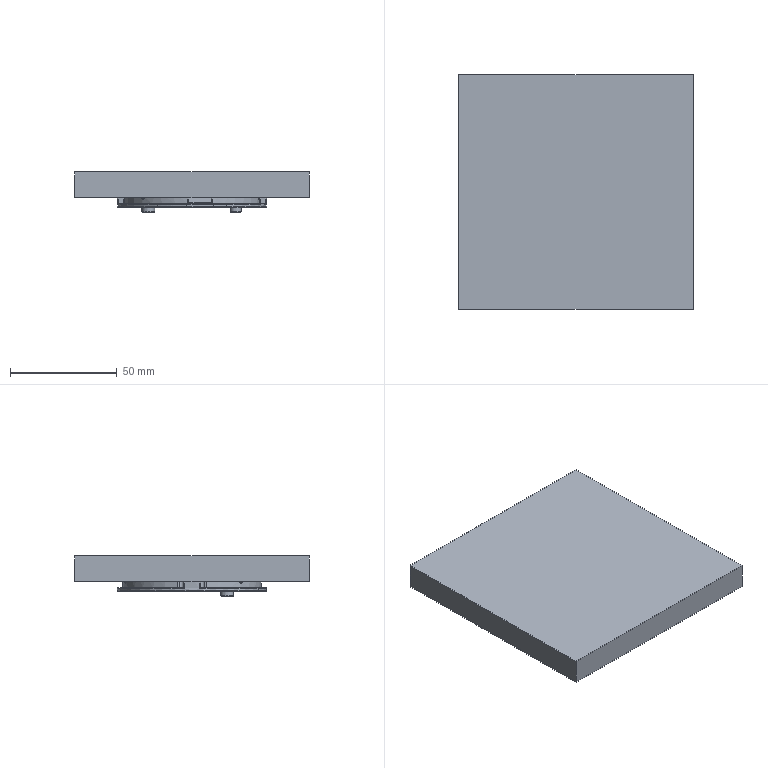NC program | NX | posted with a generic post | part box 110 x 110 x 18.8 mm
Lines 1 to 803 of 8004:
N10 G17 G21 G94 G90
(ZLEVEL_PROFILE_1 , TOOL : D10)
N12 T04 M6
N14 G54
N16 G17 G0 G90 X-39.712 Y-7.809 S9500 M3
N18 G43 Z30. H4
N20 Z5.7
N22 G94 G1 X-39.196 Y-10.314 Z5.566 F1000.
N24 X-37.85 Y-14.492 Z5.336
N26 X-36.061 Y-18.5 Z5.106
N28 X-33.85 Y-22.291 Z4.876
N30 X-31.241 Y-25.82 Z4.646
N32 X-28.266 Y-29.047 Z4.416
N34 X-24.959 Y-31.933 Z4.186
N36 X-21.36 Y-34.445 Z3.956
N38 X-17.51 Y-36.552 Z3.726
N40 X-13.455 Y-38.231 Z3.496
N42 X-11.966 Y-38.692 Z3.414
N44 X-11.87 Y-38.721 Z3.409
N46 X-11.651 Y-38.787 Z3.397
N48 X-11.428 Y-38.837 Z3.385
N50 X-8.788 Y-39.658 Z3.24
N52 X-5.617 Y-40.644 F2000.
N54 G3 X-3.659 Y-40.873 R5.367
N56 G1 X-2.722 Y-40.809
N58 X2.722 Y-40.404
N60 G3 X2.938 Y-40.393 R6.5
N62 G1 X3.03 Y-40.386
N64 G3 X-11.966 Y-38.692 R-40.5
N66 G1 X-11.87 Y-38.721
N68 G3 X-11.428 Y-38.837 R6.5
N70 G1 X-8.788 Y-39.658
N72 X-8.276 Y-39.825 Z3.231
N74 X-7.76 Y-39.984 Z3.221
N76 X-7.245 Y-40.143 Z3.212
N78 X-6.73 Y-40.302 Z3.202
N80 X-6.215 Y-40.461 Z3.193
N82 X-5.7 Y-40.62 Z3.184
N84 X-5.179 Y-40.761 Z3.174
N86 X-4.647 Y-40.849 Z3.165
N88 X-4.11 Y-40.888 Z3.155
N90 X-3.571 Y-40.872 Z3.146
N92 X-3.033 Y-40.833 Z3.136
N94 X-2.495 Y-40.793 Z3.127
N96 X-1.957 Y-40.754 Z3.118
N98 X-1.42 Y-40.714 Z3.108
N100 X-0.882 Y-40.675 Z3.099
N102 X-0.344 Y-40.635 Z3.089
N104 X0.194 Y-40.595 Z3.08
N106 X0.731 Y-40.555 Z3.071
N108 X1.269 Y-40.516 Z3.061
N110 X1.807 Y-40.477 Z3.052
N112 X2.345 Y-40.437 Z3.042
N114 X2.882 Y-40.397 Z3.033
N116 X3.42 Y-40.355 Z3.024
N118 X3.957 Y-40.306 Z3.014
N120 X4.493 Y-40.25 Z3.005
N122 X5.029 Y-40.187 Z2.995
N124 X5.563 Y-40.116 Z2.986
N126 X6.097 Y-40.038 Z2.976
N128 X6.629 Y-39.954 Z2.967
N130 X7.161 Y-39.862 Z2.958
N132 X7.691 Y-39.763 Z2.948
N134 X8.219 Y-39.657 Z2.939
N136 X8.747 Y-39.544 Z2.929
N138 X9.272 Y-39.424 Z2.92
N140 X9.796 Y-39.297 Z2.911
N142 X10.319 Y-39.163 Z2.901
N144 X10.839 Y-39.023 Z2.892
N146 X11.358 Y-38.875 Z2.882
N148 X11.874 Y-38.72 Z2.873
N150 X12.389 Y-38.559 Z2.864
N152 X12.901 Y-38.39 Z2.854
N154 X13.411 Y-38.215 Z2.845
N156 X13.918 Y-38.033 Z2.835
N158 X14.423 Y-37.845 Z2.826
N160 X14.926 Y-37.649 Z2.816
N162 X15.426 Y-37.447 Z2.807
N164 X15.923 Y-37.238 Z2.798
N166 X16.417 Y-37.023 Z2.788
N168 X16.909 Y-36.801 Z2.779
N170 X17.397 Y-36.573 Z2.769
N172 X17.883 Y-36.338 Z2.76
N174 X18.365 Y-36.097 Z2.751
N176 X18.844 Y-35.849 Z2.741
N178 X19.319 Y-35.595 Z2.732
N180 X19.792 Y-35.335 Z2.722
N182 X20.26 Y-35.068 Z2.713
N184 X20.725 Y-34.795 Z2.704
N186 X21.187 Y-34.516 Z2.694
N188 X21.644 Y-34.231 Z2.685
N190 X22.098 Y-33.94 Z2.675
N192 X22.548 Y-33.643 Z2.666
N194 X22.994 Y-33.34 Z2.656
N196 X23.436 Y-33.031 Z2.647
N198 X23.873 Y-32.716 Z2.638
N200 X24.307 Y-32.395 Z2.628
N202 X24.736 Y-32.068 Z2.619
N204 X25.161 Y-31.736 Z2.609
N206 X25.581 Y-31.398 Z2.6
N208 X25.997 Y-31.055 Z2.591
N210 X26.408 Y-30.706 Z2.581
N212 X26.814 Y-30.352 Z2.572
N214 X27.216 Y-29.992 Z2.562
N216 X27.613 Y-29.627 Z2.553
N218 X28.005 Y-29.257 Z2.544
N220 X28.392 Y-28.882 Z2.534
N222 X28.774 Y-28.501 Z2.525
N224 X29.151 Y-28.115 Z2.515
N226 X29.523 Y-27.725 Z2.506
N228 X29.889 Y-27.329 Z2.496
N230 X30.25 Y-26.929 Z2.487
N232 X30.606 Y-26.524 Z2.478
N234 X30.956 Y-26.114 Z2.468
N236 X31.301 Y-25.7 Z2.459
N238 X31.641 Y-25.281 Z2.449
N240 X31.975 Y-24.857 Z2.44
N242 X32.303 Y-24.429 Z2.431
N244 X32.625 Y-23.997 Z2.421
N246 X32.942 Y-23.561 Z2.412
N248 X33.252 Y-23.12 Z2.402
N250 X33.557 Y-22.675 Z2.393
N252 X33.856 Y-22.226 Z2.384
N254 X34.149 Y-21.774 Z2.374
N256 X34.436 Y-21.317 Z2.365
N258 X34.717 Y-20.857 Z2.355
N260 X34.991 Y-20.393 Z2.346
N262 X35.26 Y-19.925 Z2.336
N264 X35.522 Y-19.454 Z2.327
N266 X35.778 Y-18.979 Z2.318
N268 X36.027 Y-18.501 Z2.308
N270 X36.27 Y-18.02 Z2.299
N272 X36.507 Y-17.536 Z2.289
N274 X36.737 Y-17.048 Z2.28
N276 G3 X-11.966 Y-38.692 R-40.5
N278 G1 X-11.87 Y-38.721
N280 G3 X-11.428 Y-38.837 R6.5
N282 G1 X-8.788 Y-39.658
N284 X-8.276 Y-39.825 Z2.271
N286 X-7.76 Y-39.984 Z2.261
N288 X-7.245 Y-40.143 Z2.252
N290 X-6.73 Y-40.302 Z2.242
N292 X-6.215 Y-40.461 Z2.233
N294 X-5.7 Y-40.62 Z2.224
N296 X-5.179 Y-40.759 Z2.214
N298 X-4.647 Y-40.849 Z2.205
N300 X-4.11 Y-40.888 Z2.195
N302 X-3.571 Y-40.872 Z2.186
N304 X-3.033 Y-40.833 Z2.176
N306 X-2.495 Y-40.793 Z2.167
N308 X-1.957 Y-40.754 Z2.158
N310 X-1.42 Y-40.714 Z2.148
N312 X-0.882 Y-40.675 Z2.139
N314 X-0.344 Y-40.635 Z2.129
N316 X0.194 Y-40.595 Z2.12
N318 X0.731 Y-40.555 Z2.111
N320 X1.269 Y-40.516 Z2.101
N322 X1.807 Y-40.477 Z2.092
N324 X2.345 Y-40.437 Z2.082
N326 X2.882 Y-40.397 Z2.073
N328 X3.42 Y-40.355 Z2.064
N330 X3.957 Y-40.306 Z2.054
N332 X4.493 Y-40.25 Z2.045
N334 X5.029 Y-40.187 Z2.035
N336 X5.563 Y-40.116 Z2.026
N338 X6.097 Y-40.038 Z2.016
N340 X6.629 Y-39.954 Z2.007
N342 X7.161 Y-39.862 Z1.998
N344 X7.691 Y-39.763 Z1.988
N346 X8.219 Y-39.657 Z1.979
N348 X8.747 Y-39.544 Z1.969
N350 X9.272 Y-39.424 Z1.96
N352 X9.796 Y-39.297 Z1.951
N354 X10.319 Y-39.163 Z1.941
N356 X10.839 Y-39.023 Z1.932
N358 X11.358 Y-38.875 Z1.922
N360 X11.874 Y-38.72 Z1.913
N362 X12.389 Y-38.559 Z1.904
N364 X12.901 Y-38.39 Z1.894
N366 X13.411 Y-38.215 Z1.885
N368 X13.918 Y-38.033 Z1.875
N370 X14.423 Y-37.845 Z1.866
N372 X14.926 Y-37.649 Z1.856
N374 X15.426 Y-37.447 Z1.847
N376 X15.923 Y-37.238 Z1.838
N378 X16.417 Y-37.023 Z1.828
N380 X16.909 Y-36.801 Z1.819
N382 X17.397 Y-36.573 Z1.809
N384 X17.883 Y-36.338 Z1.8
N386 X18.365 Y-36.097 Z1.791
N388 X18.844 Y-35.849 Z1.781
N390 X19.319 Y-35.595 Z1.772
N392 X19.792 Y-35.335 Z1.762
N394 X20.26 Y-35.068 Z1.753
N396 X20.725 Y-34.795 Z1.744
N398 X21.187 Y-34.516 Z1.734
N400 X21.644 Y-34.231 Z1.725
N402 X22.098 Y-33.94 Z1.715
N404 X22.548 Y-33.643 Z1.706
N406 X22.994 Y-33.34 Z1.696
N408 X23.436 Y-33.031 Z1.687
N410 X23.873 Y-32.716 Z1.678
N412 X24.307 Y-32.395 Z1.668
N414 X24.736 Y-32.068 Z1.659
N416 X25.161 Y-31.736 Z1.649
N418 X25.581 Y-31.398 Z1.64
N420 X25.997 Y-31.055 Z1.631
N422 X26.408 Y-30.706 Z1.621
N424 X26.814 Y-30.352 Z1.612
N426 X27.216 Y-29.992 Z1.602
N428 X27.613 Y-29.627 Z1.593
N430 X28.005 Y-29.257 Z1.584
N432 X28.392 Y-28.882 Z1.574
N434 X28.774 Y-28.501 Z1.565
N436 X29.151 Y-28.115 Z1.555
N438 X29.523 Y-27.725 Z1.546
N440 X29.889 Y-27.329 Z1.536
N442 X30.25 Y-26.929 Z1.527
N444 X30.606 Y-26.524 Z1.518
N446 X30.956 Y-26.114 Z1.508
N448 X31.301 Y-25.7 Z1.499
N450 X31.641 Y-25.281 Z1.489
N452 X31.975 Y-24.857 Z1.48
N454 X32.303 Y-24.429 Z1.471
N456 X32.625 Y-23.997 Z1.461
N458 X32.942 Y-23.561 Z1.452
N460 X33.252 Y-23.12 Z1.442
N462 X33.557 Y-22.675 Z1.433
N464 X33.856 Y-22.226 Z1.424
N466 X34.149 Y-21.774 Z1.414
N468 X34.436 Y-21.317 Z1.405
N470 X34.717 Y-20.857 Z1.395
N472 X34.991 Y-20.393 Z1.386
N474 X35.26 Y-19.925 Z1.376
N476 X35.522 Y-19.454 Z1.367
N478 X35.778 Y-18.979 Z1.358
N480 X36.027 Y-18.501 Z1.348
N482 X36.27 Y-18.02 Z1.339
N484 X36.507 Y-17.536 Z1.329
N486 X36.737 Y-17.048 Z1.32
N488 G3 X-11.966 Y-38.692 R-40.5
N490 G1 X-11.87 Y-38.721
N492 G3 X-11.428 Y-38.837 R6.5
N494 G1 X-8.788 Y-39.658
N496 X-8.276 Y-39.825 Z1.311
N498 X-7.76 Y-39.984 Z1.301
N500 X-7.245 Y-40.143 Z1.292
N502 X-6.73 Y-40.302 Z1.282
N504 X-6.215 Y-40.461 Z1.273
N506 X-5.7 Y-40.62 Z1.264
N508 X-5.179 Y-40.759 Z1.254
N510 X-4.647 Y-40.849 Z1.245
N512 X-4.11 Y-40.888 Z1.235
N514 X-3.571 Y-40.872 Z1.226
N516 X-3.033 Y-40.833 Z1.216
N518 X-2.495 Y-40.793 Z1.207
N520 X-1.957 Y-40.754 Z1.198
N522 X-1.42 Y-40.715 Z1.188
N524 X-0.882 Y-40.675 Z1.179
N526 X-0.344 Y-40.635 Z1.169
N528 X0.194 Y-40.596 Z1.16
N530 X0.731 Y-40.555 Z1.151
N532 X1.269 Y-40.516 Z1.141
N534 X1.807 Y-40.477 Z1.132
N536 X2.345 Y-40.437 Z1.122
N538 X2.882 Y-40.397 Z1.113
N540 X3.42 Y-40.355 Z1.104
N542 X3.957 Y-40.306 Z1.094
N544 X4.493 Y-40.25 Z1.085
N546 X5.029 Y-40.187 Z1.075
N548 X5.563 Y-40.116 Z1.066
N550 X6.097 Y-40.038 Z1.056
N552 X6.629 Y-39.954 Z1.047
N554 X7.161 Y-39.862 Z1.038
N556 X7.691 Y-39.763 Z1.028
N558 X8.219 Y-39.657 Z1.019
N560 X8.747 Y-39.544 Z1.009
N562 X9.272 Y-39.424 Z1.
N564 X9.796 Y-39.297 Z0.991
N566 X10.319 Y-39.163 Z0.981
N568 X10.839 Y-39.023 Z0.972
N570 X11.358 Y-38.875 Z0.962
N572 X11.874 Y-38.72 Z0.953
N574 X12.389 Y-38.559 Z0.944
N576 X12.901 Y-38.39 Z0.934
N578 X13.411 Y-38.215 Z0.925
N580 X13.918 Y-38.033 Z0.915
N582 X14.423 Y-37.845 Z0.906
N584 X14.926 Y-37.649 Z0.896
N586 X15.426 Y-37.447 Z0.887
N588 X15.923 Y-37.239 Z0.878
N590 X16.417 Y-37.023 Z0.868
N592 X16.909 Y-36.801 Z0.859
N594 X17.397 Y-36.573 Z0.849
N596 X17.883 Y-36.338 Z0.84
N598 X18.365 Y-36.097 Z0.831
N600 X18.844 Y-35.849 Z0.821
N602 X19.319 Y-35.595 Z0.812
N604 X19.792 Y-35.335 Z0.802
N606 X20.26 Y-35.068 Z0.793
N608 X20.725 Y-34.795 Z0.784
N610 X21.187 Y-34.516 Z0.774
N612 X21.644 Y-34.231 Z0.765
N614 X22.098 Y-33.94 Z0.755
N616 X22.548 Y-33.643 Z0.746
N618 X22.994 Y-33.34 Z0.736
N620 X23.436 Y-33.031 Z0.727
N622 X23.873 Y-32.716 Z0.718
N624 X24.307 Y-32.395 Z0.708
N626 X24.736 Y-32.068 Z0.699
N628 X25.161 Y-31.736 Z0.689
N630 X25.581 Y-31.398 Z0.68
N632 X25.997 Y-31.055 Z0.671
N634 X26.408 Y-30.706 Z0.661
N636 X26.814 Y-30.352 Z0.652
N638 X27.216 Y-29.992 Z0.642
N640 X27.613 Y-29.627 Z0.633
N642 X28.005 Y-29.257 Z0.624
N644 X28.392 Y-28.882 Z0.614
N646 X28.774 Y-28.501 Z0.605
N648 X29.151 Y-28.115 Z0.595
N650 X29.523 Y-27.725 Z0.586
N652 X29.889 Y-27.329 Z0.576
N654 X30.25 Y-26.929 Z0.567
N656 X30.606 Y-26.524 Z0.558
N658 X30.956 Y-26.114 Z0.548
N660 X31.301 Y-25.7 Z0.539
N662 X31.641 Y-25.281 Z0.529
N664 X31.975 Y-24.857 Z0.52
N666 X32.303 Y-24.429 Z0.511
N668 X32.625 Y-23.997 Z0.501
N670 X32.942 Y-23.561 Z0.492
N672 X33.252 Y-23.12 Z0.482
N674 X33.557 Y-22.675 Z0.473
N676 X33.856 Y-22.227 Z0.464
N678 X34.149 Y-21.774 Z0.454
N680 X34.436 Y-21.317 Z0.445
N682 X34.717 Y-20.857 Z0.435
N684 X34.991 Y-20.393 Z0.426
N686 X35.26 Y-19.925 Z0.416
N688 X35.522 Y-19.454 Z0.407
N690 X35.778 Y-18.979 Z0.398
N692 X36.027 Y-18.501 Z0.388
N694 X36.27 Y-18.02 Z0.379
N696 X36.507 Y-17.536 Z0.369
N698 X36.737 Y-17.048 Z0.36
N700 G3 X-11.966 Y-38.692 R-40.5
N702 G1 X-11.87 Y-38.721
N704 G3 X-11.428 Y-38.837 R6.5
N706 G1 X-8.788 Y-39.658
N708 X-8.276 Y-39.825 Z0.351
N710 X-7.76 Y-39.984 Z0.341
N712 X-7.245 Y-40.143 Z0.332
N714 X-6.73 Y-40.302 Z0.322
N716 X-6.215 Y-40.461 Z0.313
N718 X-5.7 Y-40.62 Z0.304
N720 X-5.179 Y-40.759 Z0.294
N722 X-4.647 Y-40.849 Z0.285
N724 X-4.11 Y-40.888 Z0.275
N726 X-3.571 Y-40.872 Z0.266
N728 X-3.033 Y-40.833 Z0.256
N730 X-2.495 Y-40.793 Z0.247
N732 X-1.957 Y-40.754 Z0.238
N734 X-1.42 Y-40.714 Z0.228
N736 X-0.882 Y-40.675 Z0.219
N738 X-0.344 Y-40.635 Z0.209
N740 X0.194 Y-40.596 Z0.2
N742 X0.731 Y-40.556 Z0.191
N744 X1.269 Y-40.516 Z0.181
N746 X1.807 Y-40.477 Z0.172
N748 X2.345 Y-40.437 Z0.162
N750 X2.882 Y-40.397 Z0.153
N752 X3.42 Y-40.355 Z0.144
N754 X3.957 Y-40.306 Z0.134
N756 X4.493 Y-40.25 Z0.125
N758 X5.029 Y-40.187 Z0.115
N760 X5.563 Y-40.116 Z0.106
N762 X6.097 Y-40.038 Z0.096
N764 X6.629 Y-39.954 Z0.087
N766 X7.161 Y-39.862 Z0.078
N768 X7.691 Y-39.763 Z0.068
N770 X8.219 Y-39.657 Z0.059
N772 X8.747 Y-39.544 Z0.049
N774 X9.272 Y-39.424 Z0.04
N776 X9.796 Y-39.297 Z0.031
N778 X10.319 Y-39.163 Z0.021
N780 X10.839 Y-39.023 Z0.012
N782 X11.358 Y-38.875 Z0.002
N784 X11.874 Y-38.72 Z-0.007
N786 X12.389 Y-38.559 Z-0.016
N788 X12.901 Y-38.39 Z-0.026
N790 X13.411 Y-38.215 Z-0.035
N792 X13.918 Y-38.033 Z-0.045
N794 X14.423 Y-37.845 Z-0.054
N796 X14.926 Y-37.649 Z-0.064
N798 X15.426 Y-37.447 Z-0.073
N800 X15.923 Y-37.239 Z-0.082
N802 X16.417 Y-37.023 Z-0.092
N804 X16.909 Y-36.801 Z-0.101
N806 X17.397 Y-36.573 Z-0.111
N808 X17.883 Y-36.338 Z-0.12
N810 X18.365 Y-36.097 Z-0.129
N812 X18.844 Y-35.849 Z-0.139
N814 X19.319 Y-35.595 Z-0.148
N816 X19.792 Y-35.335 Z-0.158
N818 X20.26 Y-35.068 Z-0.167
N820 X20.725 Y-34.795 Z-0.176
N822 X21.187 Y-34.516 Z-0.186
N824 X21.644 Y-34.231 Z-0.195
N826 X22.098 Y-33.94 Z-0.205
N828 X22.548 Y-33.643 Z-0.214
N830 X22.994 Y-33.34 Z-0.224
N832 X23.436 Y-33.031 Z-0.233
N834 X23.873 Y-32.716 Z-0.242
N836 X24.307 Y-32.395 Z-0.252
N838 X24.736 Y-32.068 Z-0.261
N840 X25.161 Y-31.736 Z-0.271
N842 X25.581 Y-31.398 Z-0.28
N844 X25.997 Y-31.055 Z-0.289
N846 X26.408 Y-30.706 Z-0.299
N848 X26.814 Y-30.352 Z-0.308
N850 X27.216 Y-29.992 Z-0.318
N852 X27.613 Y-29.627 Z-0.327
N854 X28.005 Y-29.257 Z-0.336
N856 X28.392 Y-28.882 Z-0.346
N858 X28.774 Y-28.501 Z-0.355
N860 X29.151 Y-28.115 Z-0.365
N862 X29.523 Y-27.725 Z-0.374
N864 X29.889 Y-27.329 Z-0.384
N866 X30.25 Y-26.929 Z-0.393
N868 X30.606 Y-26.524 Z-0.402
N870 X30.956 Y-26.114 Z-0.412
N872 X31.301 Y-25.7 Z-0.421
N874 X31.641 Y-25.281 Z-0.431
N876 X31.974 Y-24.857 Z-0.44
N878 X32.303 Y-24.429 Z-0.449
N880 X32.625 Y-23.997 Z-0.459
N882 X32.942 Y-23.561 Z-0.468
N884 X33.252 Y-23.12 Z-0.478
N886 X33.557 Y-22.675 Z-0.487
N888 X33.856 Y-22.227 Z-0.496
N890 X34.149 Y-21.774 Z-0.506
N892 X34.436 Y-21.317 Z-0.515
N894 X34.717 Y-20.857 Z-0.525
N896 X34.991 Y-20.393 Z-0.534
N898 X35.26 Y-19.925 Z-0.544
N900 X35.522 Y-19.454 Z-0.553
N902 X35.778 Y-18.979 Z-0.562
N904 X36.027 Y-18.501 Z-0.572
N906 X36.27 Y-18.02 Z-0.581
N908 X36.507 Y-17.536 Z-0.591
N910 X36.737 Y-17.048 Z-0.6
N912 G3 X-11.966 Y-38.692 R-40.5
N914 G1 X-11.87 Y-38.721
N916 G3 X-11.428 Y-38.837 R6.5
N918 G1 X-5.617 Y-40.644
N920 G3 X-3.66 Y-40.873 R5.368
N922 G1 X-2.722 Y-40.809
N924 X2.722 Y-40.404
N926 G3 X2.938 Y-40.393 R6.5
N928 G1 X3.03 Y-40.386
N930 G3 X36.737 Y-17.048 R40.5
N932 G1 Z0.9
N934 G0 Z30.
N936 M5
(FLOOR_WALL_COPY , TOOL : D63)
N938 T03 M6
N940 G54
N942 G17 G0 G90 X-77.5 Y42.997 S6500 M3
N944 G43 Z30. H3
N946 Z6.6
N948 G94 G1 Z3.6 F1250.
N950 X-74.5
N952 X74.5
N954 Y12.645
N956 X-74.5
N958 Y-17.708
N960 X74.5
N962 X77.5
N964 Z6.6
N966 G0 Z30.
N968 X-77.5 Y42.997
N970 Z5.7
N972 G1 Z2.7
N974 X-74.5
N976 X74.5
N978 Y12.645
N980 X-74.5
N982 Y-17.708
N984 X74.5
N986 X77.5
N988 Z5.7
N990 G0 Z30.
N992 X-77.5 Y42.997
N994 Z4.8
N996 G1 Z1.8
N998 X-74.5
N1000 X74.5
N1002 Y12.645
N1004 X-74.5
N1006 Y-17.708
N1008 X74.5
N1010 X77.5
N1012 Z4.8
N1014 G0 Z30.
N1016 X-77.5 Y42.997
N1018 Z3.9
N1020 G1 Z0.9
N1022 X-74.5
N1024 X74.5
N1026 Y12.645
N1028 X-74.5
N1030 Y-17.708
N1032 X74.5
N1034 X77.5
N1036 Z3.9
N1038 G0 Z30.
N1040 X-77.5 Y42.997
N1042 Z3.
N1044 G1 Z0.
N1046 X-74.5
N1048 X74.5
N1050 Y12.645
N1052 X-74.5
N1054 Y-17.708
N1056 X74.5
N1058 X77.5
N1060 Z3.
N1062 G0 Z30.
N1064 M5
(DRILLING , TOOL : D4A45)
N1066 T21 M6
N1068 G54
N1070 G17 G0 G90 X-20.5 Y-16.5 S5000 M3
N1072 G43 Z30. H21
N1074 G94 G81 G98 Z-1. F250. R3.
N1076 X20.5
N1078 G80
N1080 G0 X20.5 Y-16.5 Z30.
N1082 M5
(DRILLING_COPY , TOOL : 2.5ZT)
N1084 T12 M6
N1086 G54
N1088 G17 G0 G90 X-20.5 Y-16.5 S2000 M3
N1090 G43 Z30. H12
N1092 G94 G83 G98 Z-8.251 F150. Q2. R3.
N1094 X20.5 Z-6.551
N1096 G80
N1098 G0 X20.5 Y-16.5 Z30.
N1100 M5
(FLOOR_WALL_2 , TOOL : D10)
N1102 T04 M6
N1104 G54
N1106 G17 G0 G90 X-6.271 Y40.811 S9500 M3
N1108 G43 Z30. H4
N1110 Z0.9
N1112 G94 G1 Z-0.6 F1000.
N1114 X-2.611 Y35.2
N1116 G3 X-1.719 Y34.748 R1.
N1118 G2 X29.78 Y-18.005 R34.791 F2500.
N1120 G1 X29.326 Y-18.718
N1122 G3 X24.571 Y-24.639 R-9.1
N1124 G1 X24.124 Y-23.744
N1126 G2 X13.256 Y-20.124 R8.1
N1128 X24.124 Y-23.744 R-8.1
N1130 G1 X24.571 Y-24.639
N1132 G2 X2.559 Y-34.706 R34.77
N1134 G1 X2.341 Y-34.692
N1136 X1.983 Y-34.652
N1138 X-10.235 Y-33.261
N1140 G2 X-26.016 Y-23.098 R34.662
N1142 G3 X-28.124 Y-20.479 R-8.6
N1144 G1 X-27.238 Y-20.016
N1146 G2 X-24.016 Y-9.762 R7.6
N1148 X-27.238 Y-20.016 R-7.6
N1150 G1 X-28.124 Y-20.479
N1152 G2 X-1.719 Y34.748 R34.782
N1154 G1 X-1.448 Y29.755
N1156 G2 X29.284 Y-5.47 R29.777
N1158 G3 X11.606 Y-27.441 R14.1
N1160 G2 X2.546 Y-29.683 R29.375
N1162 G1 X-9.116 Y-28.363
N1164 X-10.111 Y-28.031
N1166 X-11.436 Y-27.517
N1168 X-12.121 Y-27.213
N1170 G3 X-29.175 Y-6.026 R-13.6
N1172 G2 X-1.448 Y29.755 R29.775
N1174 G1 X-1.176 Y24.763
N1176 G2 X24.701 Y2.132 R24.777
N1178 G3 X3.196 Y-24.586 R19.1
N1180 G1 X3. Y-24.615
N1182 X2.584 Y-24.656
N1184 X-3.466 Y-23.971
N1186 G3 X-24.743 Y1.609 R18.6
N1188 G2 X-1.176 Y24.763 R24.782
N1190 G1 X-0.904 Y19.77
N1192 G2 X18.314 Y7.501 R19.767
N1194 G3 X-0.291 Y-4.312 R24.1
N1196 X-18.506 Y7.016 R23.6
N1198 G2 X-0.904 Y19.77 R19.767
N1200 G1 X-0.632 Y14.778
N1202 G2 X10.196 Y10.715 R14.749
N1204 G3 X-0.352 Y3.798 R29.1
N1206 X-10.59 Y10.328 R28.6
N1208 G2 X-0.632 Y14.778 R14.762
N1210 G1 X-0.388 Y10.284
N1212 X0.22 Y10.29
N1214 G3 X-0.407 Y9.803 R33.6
N1216 X-0.994 Y10.242 R33.1
N1218 G1 X-0.804 Y10.262
N1220 X-0.388 Y10.284
N1222 G3 X0.45 Y10.831 R1.
N1224 G1 Z0.9
N1226 G0 X-6.271 Y40.811 Z0.1
N1228 G1 Z-1.4 F1000.
N1230 X-2.611 Y35.2
N1232 G3 X-1.719 Y34.748 R1.
N1234 G2 X29.78 Y-18.005 R34.791 F2500.
N1236 G1 X29.326 Y-18.718
N1238 G3 X24.571 Y-24.639 R-9.1
N1240 G1 X24.124 Y-23.744
N1242 G2 X13.256 Y-20.124 R8.1
N1244 X24.124 Y-23.744 R-8.1
N1246 G1 X24.571 Y-24.639
N1248 G2 X2.559 Y-34.706 R34.77
N1250 G1 X2.341 Y-34.692
N1252 X1.983 Y-34.652
N1254 X-10.235 Y-33.261
N1256 G2 X-26.016 Y-23.098 R34.662
N1258 G3 X-28.124 Y-20.479 R-8.6
N1260 G1 X-27.238 Y-20.016
N1262 G2 X-24.016 Y-9.762 R7.6
N1264 X-27.238 Y-20.016 R-7.6
N1266 G1 X-28.124 Y-20.479
N1268 G2 X-1.719 Y34.748 R34.782
N1270 G1 X-1.448 Y29.755
N1272 G2 X29.284 Y-5.47 R29.777
N1274 G3 X11.606 Y-27.441 R14.1
N1276 G2 X2.546 Y-29.683 R29.375
N1278 G1 X-9.116 Y-28.363
N1280 X-10.111 Y-28.031
N1282 X-11.436 Y-27.517
N1284 X-12.121 Y-27.213
N1286 G3 X-29.175 Y-6.026 R-13.6
N1288 G2 X-1.448 Y29.755 R29.775
N1290 G1 X-1.176 Y24.763
N1292 G2 X24.701 Y2.132 R24.777
N1294 G3 X3.196 Y-24.586 R19.1
N1296 G1 X3. Y-24.615
N1298 X2.584 Y-24.656
N1300 X-3.466 Y-23.971
N1302 G3 X-24.743 Y1.609 R18.6
N1304 G2 X-1.176 Y24.763 R24.782
N1306 G1 X-0.904 Y19.77
N1308 G2 X18.314 Y7.501 R19.767
N1310 G3 X-0.291 Y-4.312 R24.1
N1312 X-18.506 Y7.016 R23.6
N1314 G2 X-0.904 Y19.77 R19.767
N1316 G1 X-0.632 Y14.778
N1318 G2 X10.196 Y10.715 R14.749
N1320 G3 X-0.352 Y3.798 R29.1
N1322 X-10.59 Y10.328 R28.6
N1324 G2 X-0.632 Y14.778 R14.762
N1326 G1 X-0.388 Y10.284
N1328 X0.22 Y10.29
N1330 G3 X-0.407 Y9.803 R33.6
N1332 X-0.994 Y10.242 R33.1
N1334 G1 X-0.804 Y10.262
N1336 X-0.388 Y10.284
N1338 G3 X0.45 Y10.831 R1.
N1340 G1 Z0.1
N1342 G0 X-6.271 Y40.811 Z-0.7
N1344 G1 Z-2.2 F1000.
N1346 X-2.611 Y35.2
N1348 G3 X-1.719 Y34.748 R1.
N1350 G2 X29.78 Y-18.005 R34.791 F2500.
N1352 G1 X29.326 Y-18.718
N1354 G3 X24.571 Y-24.639 R-9.1
N1356 G1 X24.124 Y-23.744
N1358 G2 X13.256 Y-20.124 R8.1
N1360 X24.124 Y-23.744 R-8.1
N1362 G1 X24.571 Y-24.639
N1364 G2 X2.559 Y-34.706 R34.77
N1366 G1 X2.341 Y-34.692
N1368 X1.983 Y-34.652
N1370 X-10.235 Y-33.261
N1372 G2 X-26.016 Y-23.098 R34.662
N1374 G3 X-28.124 Y-20.479 R-8.6
N1376 G1 X-27.238 Y-20.016
N1378 G2 X-24.016 Y-9.762 R7.6
N1380 X-27.238 Y-20.016 R-7.6
N1382 G1 X-28.124 Y-20.479
N1384 G2 X-1.719 Y34.748 R34.782
N1386 G1 X-1.448 Y29.755
N1388 G2 X29.284 Y-5.47 R29.777
N1390 G3 X11.606 Y-27.441 R14.1
N1392 G2 X2.546 Y-29.683 R29.375
N1394 G1 X-9.116 Y-28.363
N1396 X-10.111 Y-28.031
N1398 X-11.436 Y-27.517
N1400 X-12.121 Y-27.213
N1402 G3 X-29.175 Y-6.026 R-13.6
N1404 G2 X-1.448 Y29.755 R29.775
N1406 G1 X-1.176 Y24.763
N1408 G2 X24.701 Y2.132 R24.777
N1410 G3 X3.196 Y-24.586 R19.1
N1412 G1 X3. Y-24.615
N1414 X2.584 Y-24.656
N1416 X-3.466 Y-23.971
N1418 G3 X-24.743 Y1.609 R18.6
N1420 G2 X-1.176 Y24.763 R24.782
N1422 G1 X-0.904 Y19.77
N1424 G2 X18.314 Y7.501 R19.767
N1426 G3 X-0.291 Y-4.312 R24.1
N1428 X-18.506 Y7.016 R23.6
N1430 G2 X-0.904 Y19.77 R19.767
N1432 G1 X-0.632 Y14.778
N1434 G2 X10.196 Y10.715 R14.749
N1436 G3 X-0.352 Y3.798 R29.1
N1438 X-10.59 Y10.328 R28.6
N1440 G2 X-0.632 Y14.778 R14.762
N1442 G1 X-0.388 Y10.284
N1444 X0.22 Y10.29
N1446 G3 X-0.407 Y9.803 R33.6
N1448 X-0.994 Y10.242 R33.1
N1450 G1 X-0.804 Y10.262
N1452 X-0.388 Y10.284
N1454 G3 X0.45 Y10.831 R1.
N1456 G1 Z-0.7
N1458 G0 Z30.
(ZLEVEL_PROFILE_1_COPY , TOOL : D10)
N1460 X5.6 Y-41.625
N1462 Z-3.3
N1464 G1 X4.675 Y-40.264 F1000.
N1466 G3 X3.774 Y-39.828 R1.
N1468 G1 X3.33 Y-39.861 F1500.
N1470 G2 X2.941 Y-39.892 R40.
N1472 X-3.333 Y-35.314 R6.
N1474 G1 X-3.435 Y-34.788
N1476 G2 X-3.5 Y-33.908 R6.
N1478 G1 Y-27.25
N1480 G2 X2.5 Y-21.25 R6.
N1482 G1 X10.726
N1484 X10.743 Y-21.243
N1486 X10.75 Y-21.202
N1488 Y-11.756
N1490 X10.707 Y-11.75
N1492 X-10.706
N1494 X-10.75 Y-11.758
N1496 Y-21.197
N1498 X-10.742 Y-21.25
N1500 X-10.
N1502 G2 X-4. Y-27.25 R6.
N1504 G1 Y-32.496
N1506 G2 X-11.768 Y-38.23 R6.
N1508 X-12.211 Y-38.091 R40.
N1510 G1 X-12.655 Y-37.954
N1512 G3 X-13.63 Y-38.179 R1.
N1514 G1 X-14.828 Y-39.295
N1516 G0 X-14.825 Y-39.297 Z-4.3
N1518 G1 X-13.63 Y-38.181 F1000.
N1520 G2 X-12.656 Y-37.955 R1.
N1522 G1 X-12.211 Y-38.091 F1500.
N1524 G3 X-11.751 Y-38.235 R40.
N1526 X-4. Y-32.496 R6.
N1528 G1 Y-27.25
N1530 G3 X-10. Y-21.25 R6.
N1532 G1 X-10.741
N1534 X-10.73 Y-21.221
N1536 X-10.75 Y-21.197
N1538 Y-11.759
N1540 X-10.706 Y-11.75
N1542 X10.707
N1544 X10.75 Y-11.756
N1546 Y-21.202
N1548 X10.742 Y-21.242
N1550 X10.726 Y-21.25
N1552 X2.5
N1554 G3 X-3.5 Y-27.25 R6.
N1556 G1 Y-33.908
N1558 G3 X-3.435 Y-34.788 R6.
N1560 G1 X-3.333 Y-35.314
N1562 G3 X2.941 Y-39.892 R6.
N1564 X3.33 Y-39.861 R40.
N1566 G1 X3.774 Y-39.829
N1568 G2 X4.674 Y-40.265 R1.
N1570 G1 X5.597 Y-41.625
N1572 G0 Z30.
N1574 M5